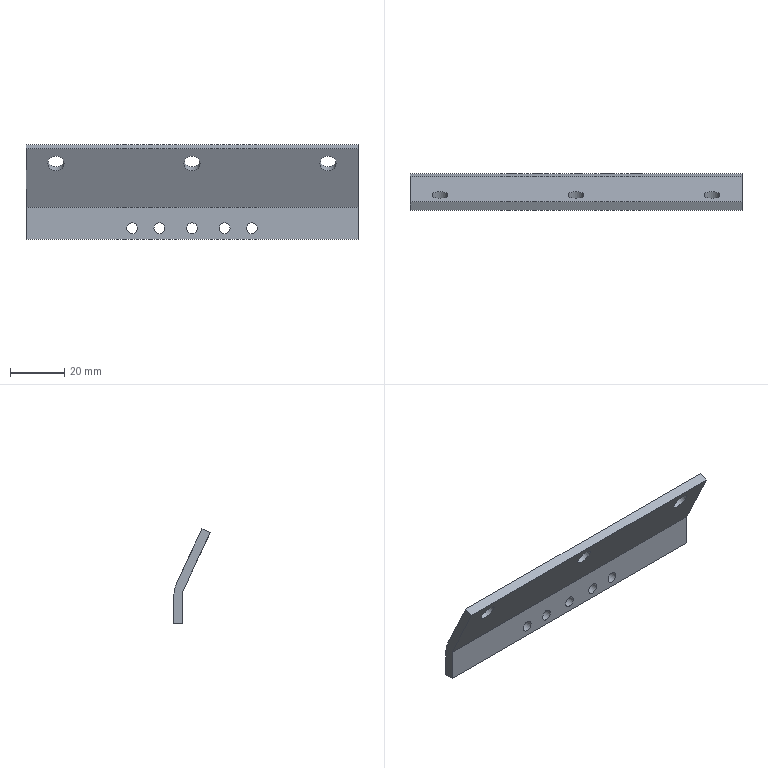Part | STEP file | 1-68.1 | 1 solid | 17 faces | box 122 x 13.367 x 34.723 mm | volume 14145 mm3 | cylinder 9 | plane 8 | commonest cylinder face diameters 4 x5 6 x3 24 x1
STEP:
#1=CARTESIAN_POINT('',(0.,0.,0.));
#2=DIRECTION('',(0.,0.,1.));
#3=DIRECTION('',(1.,0.,0.));
#4=AXIS2_PLACEMENT_3D('',#1,#2,#3);
#5=CARTESIAN_POINT('',(-61.,0.,0.));
#6=VERTEX_POINT('',#5);
#7=CARTESIAN_POINT('',(-61.,3.32,0.));
#8=VERTEX_POINT('',#7);
#9=CARTESIAN_POINT('',(-61.,0.,0.));
#10=DIRECTION('',(0.,1.,0.));
#11=VECTOR('',#10,1.);
#12=LINE('',#9,#11);
#13=CARTESIAN_POINT('',(-61.,7.314,17.361));
#14=DIRECTION('',(1.,0.,0.));
#15=DIRECTION('',(0.,1.,0.));
#16=AXIS2_PLACEMENT_3D('',#13,#14,#15);
#17=PLANE('',#16);
#18=CARTESIAN_POINT('',(-7.314,-17.361));
#19=DIRECTION('',(1.,0.));
#20=VECTOR('',#19,1.);
#21=LINE('',#18,#20);
#22=(GEOMETRIC_REPRESENTATION_CONTEXT(2)PARAMETRIC_REPRESENTATION_CONTEXT()REPRESENTATION_CONTEXT('',''));
#23=DEFINITIONAL_REPRESENTATION('',(#21),#22);
#24=PCURVE('',#17,#23);
#25=CARTESIAN_POINT('',(0.,1.66,0.));
#26=DIRECTION('',(0.,0.,-1.));
#27=DIRECTION('',(0.,1.,0.));
#28=AXIS2_PLACEMENT_3D('',#25,#26,#27);
#29=PLANE('',#28);
#30=CARTESIAN_POINT('',(-1.66,-61.));
#31=DIRECTION('',(1.,0.));
#32=VECTOR('',#31,1.);
#33=LINE('',#30,#32);
#34=(GEOMETRIC_REPRESENTATION_CONTEXT(2)PARAMETRIC_REPRESENTATION_CONTEXT()REPRESENTATION_CONTEXT('',''));
#35=DEFINITIONAL_REPRESENTATION('',(#33),#34);
#36=PCURVE('',#29,#35);
#37=SURFACE_CURVE('',#12,(#24,#36),.PCURVE_S1.);
#38=EDGE_CURVE('',#6,#8,#37,.T.);
#39=ORIENTED_EDGE('',*,*,#38,.T.);
#40=CARTESIAN_POINT('',(-61.,3.32,9.849));
#41=VERTEX_POINT('',#40);
#42=CARTESIAN_POINT('',(-61.,3.32,0.));
#43=DIRECTION('',(0.,0.,1.));
#44=VECTOR('',#43,1.);
#45=LINE('',#42,#44);
#46=CARTESIAN_POINT('',(-3.994,-17.361));
#47=DIRECTION('',(0.,1.));
#48=VECTOR('',#47,1.);
#49=LINE('',#46,#48);
#50=(GEOMETRIC_REPRESENTATION_CONTEXT(2)PARAMETRIC_REPRESENTATION_CONTEXT()REPRESENTATION_CONTEXT('',''));
#51=DEFINITIONAL_REPRESENTATION('',(#49),#50);
#52=PCURVE('',#17,#51);
#53=CARTESIAN_POINT('',(0.,3.32,4.925));
#54=DIRECTION('',(0.,1.,0.));
#55=DIRECTION('',(0.,0.,1.));
#56=AXIS2_PLACEMENT_3D('',#53,#54,#55);
#57=PLANE('',#56);
#58=CARTESIAN_POINT('',(-4.925,-61.));
#59=DIRECTION('',(1.,0.));
#60=VECTOR('',#59,1.);
#61=LINE('',#58,#60);
#62=(GEOMETRIC_REPRESENTATION_CONTEXT(2)PARAMETRIC_REPRESENTATION_CONTEXT()REPRESENTATION_CONTEXT('',''));
#63=DEFINITIONAL_REPRESENTATION('',(#61),#62);
#64=PCURVE('',#57,#63);
#65=SURFACE_CURVE('',#45,(#52,#64),.PCURVE_S1.);
#66=EDGE_CURVE('',#8,#41,#65,.T.);
#67=ORIENTED_EDGE('',*,*,#66,.T.);
#68=CARTESIAN_POINT('',(-61.,2.196,14.921));
#69=VERTEX_POINT('',#68);
#70=CARTESIAN_POINT('',(-61.,-8.68,9.849));
#71=DIRECTION('',(1.,0.,0.));
#72=DIRECTION('',(0.,1.,0.));
#73=AXIS2_PLACEMENT_3D('',#70,#71,#72);
#74=CIRCLE('',#73,12.);
#75=CARTESIAN_POINT('',(-15.994,-7.512));
#76=DIRECTION('',(1.,0.));
#77=AXIS2_PLACEMENT_2D('',#75,#76);
#78=CIRCLE('',#77,12.);
#79=(GEOMETRIC_REPRESENTATION_CONTEXT(2)PARAMETRIC_REPRESENTATION_CONTEXT()REPRESENTATION_CONTEXT('',''));
#80=DEFINITIONAL_REPRESENTATION('',(#78),#79);
#81=PCURVE('',#17,#80);
#82=CARTESIAN_POINT('',(-61.,-8.68,9.849));
#83=DIRECTION('',(1.,0.,0.));
#84=DIRECTION('',(0.,1.,0.));
#85=AXIS2_PLACEMENT_3D('',#82,#83,#84);
#86=CYLINDRICAL_SURFACE('',#85,12.);
#87=CARTESIAN_POINT('',(0.,0.));
#88=DIRECTION('',(1.,0.));
#89=VECTOR('',#88,1.);
#90=LINE('',#87,#89);
#91=(GEOMETRIC_REPRESENTATION_CONTEXT(2)PARAMETRIC_REPRESENTATION_CONTEXT()REPRESENTATION_CONTEXT('',''));
#92=DEFINITIONAL_REPRESENTATION('',(#90),#91);
#93=PCURVE('',#86,#92);
#94=SURFACE_CURVE('',#74,(#81,#93),.PCURVE_S1.);
#95=EDGE_CURVE('',#41,#69,#94,.T.);
#96=ORIENTED_EDGE('',*,*,#95,.T.);
#97=CARTESIAN_POINT('',(-61.,-7.038,34.723));
#98=VERTEX_POINT('',#97);
#99=CARTESIAN_POINT('',(-61.,2.196,14.921));
#100=DIRECTION('',(0.,-0.4226,0.9063));
#101=VECTOR('',#100,1.);
#102=LINE('',#99,#101);
#103=CARTESIAN_POINT('',(-5.118,-2.441));
#104=DIRECTION('',(-0.4226,0.9063));
#105=VECTOR('',#104,1.);
#106=LINE('',#103,#105);
#107=(GEOMETRIC_REPRESENTATION_CONTEXT(2)PARAMETRIC_REPRESENTATION_CONTEXT()REPRESENTATION_CONTEXT('',''));
#108=DEFINITIONAL_REPRESENTATION('',(#106),#107);
#109=PCURVE('',#17,#108);
#110=CARTESIAN_POINT('',(0.,-2.421,24.822));
#111=DIRECTION('',(0.,0.9063,0.4226));
#112=DIRECTION('',(0.,-0.4226,0.9063));
#113=AXIS2_PLACEMENT_3D('',#110,#111,#112);
#114=PLANE('',#113);
#115=CARTESIAN_POINT('',(-10.925,-61.));
#116=DIRECTION('',(1.,0.));
#117=VECTOR('',#116,1.);
#118=LINE('',#115,#117);
#119=(GEOMETRIC_REPRESENTATION_CONTEXT(2)PARAMETRIC_REPRESENTATION_CONTEXT()REPRESENTATION_CONTEXT('',''));
#120=DEFINITIONAL_REPRESENTATION('',(#118),#119);
#121=PCURVE('',#114,#120);
#122=SURFACE_CURVE('',#102,(#109,#121),.PCURVE_S1.);
#123=EDGE_CURVE('',#69,#98,#122,.T.);
#124=ORIENTED_EDGE('',*,*,#123,.T.);
#125=CARTESIAN_POINT('',(-61.,-10.047,33.32));
#126=VERTEX_POINT('',#125);
#127=CARTESIAN_POINT('',(-61.,-7.038,34.723));
#128=DIRECTION('',(0.,-0.9063,-0.4226));
#129=VECTOR('',#128,1.);
#130=LINE('',#127,#129);
#131=CARTESIAN_POINT('',(-14.352,17.361));
#132=DIRECTION('',(-0.9063,-0.4226));
#133=VECTOR('',#132,1.);
#134=LINE('',#131,#133);
#135=(GEOMETRIC_REPRESENTATION_CONTEXT(2)PARAMETRIC_REPRESENTATION_CONTEXT()REPRESENTATION_CONTEXT('',''));
#136=DEFINITIONAL_REPRESENTATION('',(#134),#135);
#137=PCURVE('',#17,#136);
#138=CARTESIAN_POINT('',(0.,-8.543,34.021));
#139=DIRECTION('',(0.,-0.4226,0.9063));
#140=DIRECTION('',(0.,-0.9063,-0.4226));
#141=AXIS2_PLACEMENT_3D('',#138,#139,#140);
#142=PLANE('',#141);
#143=CARTESIAN_POINT('',(-1.66,-61.));
#144=DIRECTION('',(1.,0.));
#145=VECTOR('',#144,1.);
#146=LINE('',#143,#145);
#147=(GEOMETRIC_REPRESENTATION_CONTEXT(2)PARAMETRIC_REPRESENTATION_CONTEXT()REPRESENTATION_CONTEXT('',''));
#148=DEFINITIONAL_REPRESENTATION('',(#146),#147);
#149=PCURVE('',#142,#148);
#150=SURFACE_CURVE('',#130,(#137,#149),.PCURVE_S1.);
#151=EDGE_CURVE('',#98,#126,#150,.T.);
#152=ORIENTED_EDGE('',*,*,#151,.T.);
#153=CARTESIAN_POINT('',(-61.,0.,11.774));
#154=VERTEX_POINT('',#153);
#155=CARTESIAN_POINT('',(-61.,-10.047,33.32));
#156=DIRECTION('',(0.,0.4226,-0.9063));
#157=VECTOR('',#156,1.);
#158=LINE('',#155,#157);
#159=CARTESIAN_POINT('',(-17.361,15.958));
#160=DIRECTION('',(0.4226,-0.9063));
#161=VECTOR('',#160,1.);
#162=LINE('',#159,#161);
#163=(GEOMETRIC_REPRESENTATION_CONTEXT(2)PARAMETRIC_REPRESENTATION_CONTEXT()REPRESENTATION_CONTEXT('',''));
#164=DEFINITIONAL_REPRESENTATION('',(#162),#163);
#165=PCURVE('',#17,#164);
#166=CARTESIAN_POINT('',(0.,-5.024,22.547));
#167=DIRECTION('',(0.,-0.9063,-0.4226));
#168=DIRECTION('',(0.,0.4226,-0.9063));
#169=AXIS2_PLACEMENT_3D('',#166,#167,#168);
#170=PLANE('',#169);
#171=CARTESIAN_POINT('',(-11.887,-61.));
#172=DIRECTION('',(1.,0.));
#173=VECTOR('',#172,1.);
#174=LINE('',#171,#173);
#175=(GEOMETRIC_REPRESENTATION_CONTEXT(2)PARAMETRIC_REPRESENTATION_CONTEXT()REPRESENTATION_CONTEXT('',''));
#176=DEFINITIONAL_REPRESENTATION('',(#174),#175);
#177=PCURVE('',#170,#176);
#178=SURFACE_CURVE('',#158,(#165,#177),.PCURVE_S1.);
#179=EDGE_CURVE('',#126,#154,#178,.T.);
#180=ORIENTED_EDGE('',*,*,#179,.T.);
#181=CARTESIAN_POINT('',(-61.,0.,11.774));
#182=DIRECTION('',(0.,0.,-1.));
#183=VECTOR('',#182,1.);
#184=LINE('',#181,#183);
#185=CARTESIAN_POINT('',(-7.314,-5.588));
#186=DIRECTION('',(0.,-1.));
#187=VECTOR('',#186,1.);
#188=LINE('',#185,#187);
#189=(GEOMETRIC_REPRESENTATION_CONTEXT(2)PARAMETRIC_REPRESENTATION_CONTEXT()REPRESENTATION_CONTEXT('',''));
#190=DEFINITIONAL_REPRESENTATION('',(#188),#189);
#191=PCURVE('',#17,#190);
#192=CARTESIAN_POINT('',(0.,0.,5.887));
#193=DIRECTION('',(0.,-1.,0.));
#194=DIRECTION('',(0.,0.,-1.));
#195=AXIS2_PLACEMENT_3D('',#192,#193,#194);
#196=PLANE('',#195);
#197=CARTESIAN_POINT('',(-5.887,-61.));
#198=DIRECTION('',(1.,0.));
#199=VECTOR('',#198,1.);
#200=LINE('',#197,#199);
#201=(GEOMETRIC_REPRESENTATION_CONTEXT(2)PARAMETRIC_REPRESENTATION_CONTEXT()REPRESENTATION_CONTEXT('',''));
#202=DEFINITIONAL_REPRESENTATION('',(#200),#201);
#203=PCURVE('',#196,#202);
#204=SURFACE_CURVE('',#184,(#191,#203),.PCURVE_S1.);
#205=EDGE_CURVE('',#154,#6,#204,.T.);
#206=ORIENTED_EDGE('',*,*,#205,.T.);
#207=EDGE_LOOP('',(#39,#67,#96,#124,#152,#180,#206));
#208=FACE_BOUND('',#207,.F.);
#209=ADVANCED_FACE('',(#208),#17,.F.);
#210=CARTESIAN_POINT('',(61.,0.,0.));
#211=VERTEX_POINT('',#210);
#212=CARTESIAN_POINT('',(61.,3.32,0.));
#213=VERTEX_POINT('',#212);
#214=CARTESIAN_POINT('',(61.,0.,0.));
#215=DIRECTION('',(0.,1.,0.));
#216=VECTOR('',#215,1.);
#217=LINE('',#214,#216);
#218=CARTESIAN_POINT('',(61.,7.314,17.361));
#219=DIRECTION('',(1.,0.,0.));
#220=DIRECTION('',(0.,1.,0.));
#221=AXIS2_PLACEMENT_3D('',#218,#219,#220);
#222=PLANE('',#221);
#223=CARTESIAN_POINT('',(-7.314,-17.361));
#224=DIRECTION('',(1.,0.));
#225=VECTOR('',#224,1.);
#226=LINE('',#223,#225);
#227=(GEOMETRIC_REPRESENTATION_CONTEXT(2)PARAMETRIC_REPRESENTATION_CONTEXT()REPRESENTATION_CONTEXT('',''));
#228=DEFINITIONAL_REPRESENTATION('',(#226),#227);
#229=PCURVE('',#222,#228);
#230=CARTESIAN_POINT('',(-1.66,61.));
#231=DIRECTION('',(1.,0.));
#232=VECTOR('',#231,1.);
#233=LINE('',#230,#232);
#234=(GEOMETRIC_REPRESENTATION_CONTEXT(2)PARAMETRIC_REPRESENTATION_CONTEXT()REPRESENTATION_CONTEXT('',''));
#235=DEFINITIONAL_REPRESENTATION('',(#233),#234);
#236=PCURVE('',#29,#235);
#237=SURFACE_CURVE('',#217,(#229,#236),.PCURVE_S1.);
#238=EDGE_CURVE('',#211,#213,#237,.T.);
#239=ORIENTED_EDGE('',*,*,#238,.T.);
#240=CARTESIAN_POINT('',(61.,3.32,9.849));
#241=VERTEX_POINT('',#240);
#242=CARTESIAN_POINT('',(61.,3.32,0.));
#243=DIRECTION('',(0.,0.,1.));
#244=VECTOR('',#243,1.);
#245=LINE('',#242,#244);
#246=CARTESIAN_POINT('',(-3.994,-17.361));
#247=DIRECTION('',(0.,1.));
#248=VECTOR('',#247,1.);
#249=LINE('',#246,#248);
#250=(GEOMETRIC_REPRESENTATION_CONTEXT(2)PARAMETRIC_REPRESENTATION_CONTEXT()REPRESENTATION_CONTEXT('',''));
#251=DEFINITIONAL_REPRESENTATION('',(#249),#250);
#252=PCURVE('',#222,#251);
#253=CARTESIAN_POINT('',(-4.925,61.));
#254=DIRECTION('',(1.,0.));
#255=VECTOR('',#254,1.);
#256=LINE('',#253,#255);
#257=(GEOMETRIC_REPRESENTATION_CONTEXT(2)PARAMETRIC_REPRESENTATION_CONTEXT()REPRESENTATION_CONTEXT('',''));
#258=DEFINITIONAL_REPRESENTATION('',(#256),#257);
#259=PCURVE('',#57,#258);
#260=SURFACE_CURVE('',#245,(#252,#259),.PCURVE_S1.);
#261=EDGE_CURVE('',#213,#241,#260,.T.);
#262=ORIENTED_EDGE('',*,*,#261,.T.);
#263=CARTESIAN_POINT('',(61.,2.196,14.921));
#264=VERTEX_POINT('',#263);
#265=CARTESIAN_POINT('',(61.,-8.68,9.849));
#266=DIRECTION('',(1.,0.,0.));
#267=DIRECTION('',(0.,1.,0.));
#268=AXIS2_PLACEMENT_3D('',#265,#266,#267);
#269=CIRCLE('',#268,12.);
#270=CARTESIAN_POINT('',(-15.994,-7.512));
#271=DIRECTION('',(1.,0.));
#272=AXIS2_PLACEMENT_2D('',#270,#271);
#273=CIRCLE('',#272,12.);
#274=(GEOMETRIC_REPRESENTATION_CONTEXT(2)PARAMETRIC_REPRESENTATION_CONTEXT()REPRESENTATION_CONTEXT('',''));
#275=DEFINITIONAL_REPRESENTATION('',(#273),#274);
#276=PCURVE('',#222,#275);
#277=CARTESIAN_POINT('',(0.,122.));
#278=DIRECTION('',(1.,0.));
#279=VECTOR('',#278,1.);
#280=LINE('',#277,#279);
#281=(GEOMETRIC_REPRESENTATION_CONTEXT(2)PARAMETRIC_REPRESENTATION_CONTEXT()REPRESENTATION_CONTEXT('',''));
#282=DEFINITIONAL_REPRESENTATION('',(#280),#281);
#283=PCURVE('',#86,#282);
#284=SURFACE_CURVE('',#269,(#276,#283),.PCURVE_S1.);
#285=EDGE_CURVE('',#241,#264,#284,.T.);
#286=ORIENTED_EDGE('',*,*,#285,.T.);
#287=CARTESIAN_POINT('',(61.,-7.038,34.723));
#288=VERTEX_POINT('',#287);
#289=CARTESIAN_POINT('',(61.,2.196,14.921));
#290=DIRECTION('',(0.,-0.4226,0.9063));
#291=VECTOR('',#290,1.);
#292=LINE('',#289,#291);
#293=CARTESIAN_POINT('',(-5.118,-2.441));
#294=DIRECTION('',(-0.4226,0.9063));
#295=VECTOR('',#294,1.);
#296=LINE('',#293,#295);
#297=(GEOMETRIC_REPRESENTATION_CONTEXT(2)PARAMETRIC_REPRESENTATION_CONTEXT()REPRESENTATION_CONTEXT('',''));
#298=DEFINITIONAL_REPRESENTATION('',(#296),#297);
#299=PCURVE('',#222,#298);
#300=CARTESIAN_POINT('',(-10.925,61.));
#301=DIRECTION('',(1.,0.));
#302=VECTOR('',#301,1.);
#303=LINE('',#300,#302);
#304=(GEOMETRIC_REPRESENTATION_CONTEXT(2)PARAMETRIC_REPRESENTATION_CONTEXT()REPRESENTATION_CONTEXT('',''));
#305=DEFINITIONAL_REPRESENTATION('',(#303),#304);
#306=PCURVE('',#114,#305);
#307=SURFACE_CURVE('',#292,(#299,#306),.PCURVE_S1.);
#308=EDGE_CURVE('',#264,#288,#307,.T.);
#309=ORIENTED_EDGE('',*,*,#308,.T.);
#310=CARTESIAN_POINT('',(61.,-10.047,33.32));
#311=VERTEX_POINT('',#310);
#312=CARTESIAN_POINT('',(61.,-7.038,34.723));
#313=DIRECTION('',(0.,-0.9063,-0.4226));
#314=VECTOR('',#313,1.);
#315=LINE('',#312,#314);
#316=CARTESIAN_POINT('',(-14.352,17.361));
#317=DIRECTION('',(-0.9063,-0.4226));
#318=VECTOR('',#317,1.);
#319=LINE('',#316,#318);
#320=(GEOMETRIC_REPRESENTATION_CONTEXT(2)PARAMETRIC_REPRESENTATION_CONTEXT()REPRESENTATION_CONTEXT('',''));
#321=DEFINITIONAL_REPRESENTATION('',(#319),#320);
#322=PCURVE('',#222,#321);
#323=CARTESIAN_POINT('',(-1.66,61.));
#324=DIRECTION('',(1.,0.));
#325=VECTOR('',#324,1.);
#326=LINE('',#323,#325);
#327=(GEOMETRIC_REPRESENTATION_CONTEXT(2)PARAMETRIC_REPRESENTATION_CONTEXT()REPRESENTATION_CONTEXT('',''));
#328=DEFINITIONAL_REPRESENTATION('',(#326),#327);
#329=PCURVE('',#142,#328);
#330=SURFACE_CURVE('',#315,(#322,#329),.PCURVE_S1.);
#331=EDGE_CURVE('',#288,#311,#330,.T.);
#332=ORIENTED_EDGE('',*,*,#331,.T.);
#333=CARTESIAN_POINT('',(61.,0.,11.774));
#334=VERTEX_POINT('',#333);
#335=CARTESIAN_POINT('',(61.,-10.047,33.32));
#336=DIRECTION('',(0.,0.4226,-0.9063));
#337=VECTOR('',#336,1.);
#338=LINE('',#335,#337);
#339=CARTESIAN_POINT('',(-17.361,15.958));
#340=DIRECTION('',(0.4226,-0.9063));
#341=VECTOR('',#340,1.);
#342=LINE('',#339,#341);
#343=(GEOMETRIC_REPRESENTATION_CONTEXT(2)PARAMETRIC_REPRESENTATION_CONTEXT()REPRESENTATION_CONTEXT('',''));
#344=DEFINITIONAL_REPRESENTATION('',(#342),#343);
#345=PCURVE('',#222,#344);
#346=CARTESIAN_POINT('',(-11.887,61.));
#347=DIRECTION('',(1.,0.));
#348=VECTOR('',#347,1.);
#349=LINE('',#346,#348);
#350=(GEOMETRIC_REPRESENTATION_CONTEXT(2)PARAMETRIC_REPRESENTATION_CONTEXT()REPRESENTATION_CONTEXT('',''));
#351=DEFINITIONAL_REPRESENTATION('',(#349),#350);
#352=PCURVE('',#170,#351);
#353=SURFACE_CURVE('',#338,(#345,#352),.PCURVE_S1.);
#354=EDGE_CURVE('',#311,#334,#353,.T.);
#355=ORIENTED_EDGE('',*,*,#354,.T.);
#356=CARTESIAN_POINT('',(61.,0.,11.774));
#357=DIRECTION('',(0.,0.,-1.));
#358=VECTOR('',#357,1.);
#359=LINE('',#356,#358);
#360=CARTESIAN_POINT('',(-7.314,-5.588));
#361=DIRECTION('',(0.,-1.));
#362=VECTOR('',#361,1.);
#363=LINE('',#360,#362);
#364=(GEOMETRIC_REPRESENTATION_CONTEXT(2)PARAMETRIC_REPRESENTATION_CONTEXT()REPRESENTATION_CONTEXT('',''));
#365=DEFINITIONAL_REPRESENTATION('',(#363),#364);
#366=PCURVE('',#222,#365);
#367=CARTESIAN_POINT('',(-5.887,61.));
#368=DIRECTION('',(1.,0.));
#369=VECTOR('',#368,1.);
#370=LINE('',#367,#369);
#371=(GEOMETRIC_REPRESENTATION_CONTEXT(2)PARAMETRIC_REPRESENTATION_CONTEXT()REPRESENTATION_CONTEXT('',''));
#372=DEFINITIONAL_REPRESENTATION('',(#370),#371);
#373=PCURVE('',#196,#372);
#374=SURFACE_CURVE('',#359,(#366,#373),.PCURVE_S1.);
#375=EDGE_CURVE('',#334,#211,#374,.T.);
#376=ORIENTED_EDGE('',*,*,#375,.T.);
#377=EDGE_LOOP('',(#239,#262,#286,#309,#332,#355,#376));
#378=FACE_BOUND('',#377,.T.);
#379=ADVANCED_FACE('',(#378),#222,.T.);
#380=ORIENTED_EDGE('',*,*,#38,.T.);
#381=CARTESIAN_POINT('',(-61.,3.32,0.));
#382=DIRECTION('',(1.,0.,0.));
#383=VECTOR('',#382,1.);
#384=LINE('',#381,#383);
#385=CARTESIAN_POINT('',(1.66,-61.));
#386=DIRECTION('',(0.,1.));
#387=VECTOR('',#386,1.);
#388=LINE('',#385,#387);
#389=(GEOMETRIC_REPRESENTATION_CONTEXT(2)PARAMETRIC_REPRESENTATION_CONTEXT()REPRESENTATION_CONTEXT('',''));
#390=DEFINITIONAL_REPRESENTATION('',(#388),#389);
#391=PCURVE('',#29,#390);
#392=CARTESIAN_POINT('',(-4.925,-61.));
#393=DIRECTION('',(0.,1.));
#394=VECTOR('',#393,1.);
#395=LINE('',#392,#394);
#396=(GEOMETRIC_REPRESENTATION_CONTEXT(2)PARAMETRIC_REPRESENTATION_CONTEXT()REPRESENTATION_CONTEXT('',''));
#397=DEFINITIONAL_REPRESENTATION('',(#395),#396);
#398=PCURVE('',#57,#397);
#399=SURFACE_CURVE('',#384,(#391,#398),.PCURVE_S1.);
#400=EDGE_CURVE('',#8,#213,#399,.T.);
#401=ORIENTED_EDGE('',*,*,#400,.T.);
#402=ORIENTED_EDGE('',*,*,#238,.F.);
#403=CARTESIAN_POINT('',(-61.,0.,0.));
#404=DIRECTION('',(1.,0.,0.));
#405=VECTOR('',#404,1.);
#406=LINE('',#403,#405);
#407=CARTESIAN_POINT('',(-1.66,-61.));
#408=DIRECTION('',(0.,1.));
#409=VECTOR('',#408,1.);
#410=LINE('',#407,#409);
#411=(GEOMETRIC_REPRESENTATION_CONTEXT(2)PARAMETRIC_REPRESENTATION_CONTEXT()REPRESENTATION_CONTEXT('',''));
#412=DEFINITIONAL_REPRESENTATION('',(#410),#411);
#413=PCURVE('',#29,#412);
#414=CARTESIAN_POINT('',(5.887,-61.));
#415=DIRECTION('',(0.,1.));
#416=VECTOR('',#415,1.);
#417=LINE('',#414,#416);
#418=(GEOMETRIC_REPRESENTATION_CONTEXT(2)PARAMETRIC_REPRESENTATION_CONTEXT()REPRESENTATION_CONTEXT('',''));
#419=DEFINITIONAL_REPRESENTATION('',(#417),#418);
#420=PCURVE('',#196,#419);
#421=SURFACE_CURVE('',#406,(#413,#420),.PCURVE_S1.);
#422=EDGE_CURVE('',#6,#211,#421,.T.);
#423=ORIENTED_EDGE('',*,*,#422,.F.);
#424=EDGE_LOOP('',(#380,#401,#402,#423));
#425=FACE_BOUND('',#424,.T.);
#426=ADVANCED_FACE('',(#425),#29,.T.);
#427=ORIENTED_EDGE('',*,*,#95,.T.);
#428=CARTESIAN_POINT('',(-61.,2.196,14.921));
#429=DIRECTION('',(1.,0.,0.));
#430=VECTOR('',#429,1.);
#431=LINE('',#428,#430);
#432=CARTESIAN_POINT('',(0.4363,0.));
#433=DIRECTION('',(0.,1.));
#434=VECTOR('',#433,1.);
#435=LINE('',#432,#434);
#436=(GEOMETRIC_REPRESENTATION_CONTEXT(2)PARAMETRIC_REPRESENTATION_CONTEXT()REPRESENTATION_CONTEXT('',''));
#437=DEFINITIONAL_REPRESENTATION('',(#435),#436);
#438=PCURVE('',#86,#437);
#439=CARTESIAN_POINT('',(-10.925,-61.));
#440=DIRECTION('',(0.,1.));
#441=VECTOR('',#440,1.);
#442=LINE('',#439,#441);
#443=(GEOMETRIC_REPRESENTATION_CONTEXT(2)PARAMETRIC_REPRESENTATION_CONTEXT()REPRESENTATION_CONTEXT('',''));
#444=DEFINITIONAL_REPRESENTATION('',(#442),#443);
#445=PCURVE('',#114,#444);
#446=SURFACE_CURVE('',#431,(#438,#445),.PCURVE_S1.);
#447=EDGE_CURVE('',#69,#264,#446,.T.);
#448=ORIENTED_EDGE('',*,*,#447,.T.);
#449=ORIENTED_EDGE('',*,*,#285,.F.);
#450=CARTESIAN_POINT('',(-61.,3.32,9.849));
#451=DIRECTION('',(1.,0.,0.));
#452=VECTOR('',#451,1.);
#453=LINE('',#450,#452);
#454=CARTESIAN_POINT('',(0.,0.));
#455=DIRECTION('',(0.,1.));
#456=VECTOR('',#455,1.);
#457=LINE('',#454,#456);
#458=(GEOMETRIC_REPRESENTATION_CONTEXT(2)PARAMETRIC_REPRESENTATION_CONTEXT()REPRESENTATION_CONTEXT('',''));
#459=DEFINITIONAL_REPRESENTATION('',(#457),#458);
#460=PCURVE('',#86,#459);
#461=CARTESIAN_POINT('',(4.925,-61.));
#462=DIRECTION('',(0.,1.));
#463=VECTOR('',#462,1.);
#464=LINE('',#461,#463);
#465=(GEOMETRIC_REPRESENTATION_CONTEXT(2)PARAMETRIC_REPRESENTATION_CONTEXT()REPRESENTATION_CONTEXT('',''));
#466=DEFINITIONAL_REPRESENTATION('',(#464),#465);
#467=PCURVE('',#57,#466);
#468=SURFACE_CURVE('',#453,(#460,#467),.PCURVE_S1.);
#469=EDGE_CURVE('',#41,#241,#468,.T.);
#470=ORIENTED_EDGE('',*,*,#469,.F.);
#471=EDGE_LOOP('',(#427,#448,#449,#470));
#472=FACE_BOUND('',#471,.T.);
#473=ADVANCED_FACE('',(#472),#86,.T.);
#474=ORIENTED_EDGE('',*,*,#151,.T.);
#475=CARTESIAN_POINT('',(-61.,-10.047,33.32));
#476=DIRECTION('',(1.,0.,0.));
#477=VECTOR('',#476,1.);
#478=LINE('',#475,#477);
#479=CARTESIAN_POINT('',(1.66,-61.));
#480=DIRECTION('',(0.,1.));
#481=VECTOR('',#480,1.);
#482=LINE('',#479,#481);
#483=(GEOMETRIC_REPRESENTATION_CONTEXT(2)PARAMETRIC_REPRESENTATION_CONTEXT()REPRESENTATION_CONTEXT('',''));
#484=DEFINITIONAL_REPRESENTATION('',(#482),#483);
#485=PCURVE('',#142,#484);
#486=CARTESIAN_POINT('',(-11.887,-61.));
#487=DIRECTION('',(0.,1.));
#488=VECTOR('',#487,1.);
#489=LINE('',#486,#488);
#490=(GEOMETRIC_REPRESENTATION_CONTEXT(2)PARAMETRIC_REPRESENTATION_CONTEXT()REPRESENTATION_CONTEXT('',''));
#491=DEFINITIONAL_REPRESENTATION('',(#489),#490);
#492=PCURVE('',#170,#491);
#493=SURFACE_CURVE('',#478,(#485,#492),.PCURVE_S1.);
#494=EDGE_CURVE('',#126,#311,#493,.T.);
#495=ORIENTED_EDGE('',*,*,#494,.T.);
#496=ORIENTED_EDGE('',*,*,#331,.F.);
#497=CARTESIAN_POINT('',(-61.,-7.038,34.723));
#498=DIRECTION('',(1.,0.,0.));
#499=VECTOR('',#498,1.);
#500=LINE('',#497,#499);
#501=CARTESIAN_POINT('',(-1.66,-61.));
#502=DIRECTION('',(0.,1.));
#503=VECTOR('',#502,1.);
#504=LINE('',#501,#503);
#505=(GEOMETRIC_REPRESENTATION_CONTEXT(2)PARAMETRIC_REPRESENTATION_CONTEXT()REPRESENTATION_CONTEXT('',''));
#506=DEFINITIONAL_REPRESENTATION('',(#504),#505);
#507=PCURVE('',#142,#506);
#508=CARTESIAN_POINT('',(10.925,-61.));
#509=DIRECTION('',(0.,1.));
#510=VECTOR('',#509,1.);
#511=LINE('',#508,#510);
#512=(GEOMETRIC_REPRESENTATION_CONTEXT(2)PARAMETRIC_REPRESENTATION_CONTEXT()REPRESENTATION_CONTEXT('',''));
#513=DEFINITIONAL_REPRESENTATION('',(#511),#512);
#514=PCURVE('',#114,#513);
#515=SURFACE_CURVE('',#500,(#507,#514),.PCURVE_S1.);
#516=EDGE_CURVE('',#98,#288,#515,.T.);
#517=ORIENTED_EDGE('',*,*,#516,.F.);
#518=EDGE_LOOP('',(#474,#495,#496,#517));
#519=FACE_BOUND('',#518,.T.);
#520=ADVANCED_FACE('',(#519),#142,.T.);
#521=ORIENTED_EDGE('',*,*,#123,.T.);
#522=ORIENTED_EDGE('',*,*,#516,.T.);
#523=ORIENTED_EDGE('',*,*,#308,.F.);
#524=ORIENTED_EDGE('',*,*,#447,.F.);
#525=EDGE_LOOP('',(#521,#522,#523,#524));
#526=FACE_BOUND('',#525,.T.);
#527=CARTESIAN_POINT('',(47.,-4.502,29.285));
#528=VERTEX_POINT('',#527);
#529=CARTESIAN_POINT('',(50.,-4.502,29.285));
#530=DIRECTION('',(0.,0.9063,0.4226));
#531=DIRECTION('',(-1.,0.,0.));
#532=AXIS2_PLACEMENT_3D('',#529,#530,#531);
#533=CIRCLE('',#532,3.);
#534=CARTESIAN_POINT('',(4.925,50.));
#535=DIRECTION('',(0.,-1.));
#536=AXIS2_PLACEMENT_2D('',#534,#535);
#537=CIRCLE('',#536,3.);
#538=(GEOMETRIC_REPRESENTATION_CONTEXT(2)PARAMETRIC_REPRESENTATION_CONTEXT()REPRESENTATION_CONTEXT('',''));
#539=DEFINITIONAL_REPRESENTATION('',(#537),#538);
#540=PCURVE('',#114,#539);
#541=CARTESIAN_POINT('',(50.,-59.787,3.505));
#542=DIRECTION('',(0.,0.9063,0.4226));
#543=DIRECTION('',(-1.,0.,0.));
#544=AXIS2_PLACEMENT_3D('',#541,#542,#543);
#545=CYLINDRICAL_SURFACE('',#544,3.);
#546=CARTESIAN_POINT('',(0.,61.));
#547=DIRECTION('',(1.,0.));
#548=VECTOR('',#547,1.);
#549=LINE('',#546,#548);
#550=(GEOMETRIC_REPRESENTATION_CONTEXT(2)PARAMETRIC_REPRESENTATION_CONTEXT()REPRESENTATION_CONTEXT('',''));
#551=DEFINITIONAL_REPRESENTATION('',(#549),#550);
#552=PCURVE('',#545,#551);
#553=SURFACE_CURVE('',#533,(#540,#552),.PCURVE_S1.);
#554=EDGE_CURVE('',#528,#528,#553,.T.);
#555=ORIENTED_EDGE('',*,*,#554,.F.);
#556=EDGE_LOOP('',(#555));
#557=FACE_BOUND('',#556,.T.);
#558=CARTESIAN_POINT('',(-3.,-4.502,29.285));
#559=VERTEX_POINT('',#558);
#560=CARTESIAN_POINT('',(0.,-4.502,29.285));
#561=DIRECTION('',(0.,0.9063,0.4226));
#562=DIRECTION('',(-1.,0.,0.));
#563=AXIS2_PLACEMENT_3D('',#560,#561,#562);
#564=CIRCLE('',#563,3.);
#565=CARTESIAN_POINT('',(4.925,0.));
#566=DIRECTION('',(0.,-1.));
#567=AXIS2_PLACEMENT_2D('',#565,#566);
#568=CIRCLE('',#567,3.);
#569=(GEOMETRIC_REPRESENTATION_CONTEXT(2)PARAMETRIC_REPRESENTATION_CONTEXT()REPRESENTATION_CONTEXT('',''));
#570=DEFINITIONAL_REPRESENTATION('',(#568),#569);
#571=PCURVE('',#114,#570);
#572=CARTESIAN_POINT('',(0.,-59.787,3.505));
#573=DIRECTION('',(0.,0.9063,0.4226));
#574=DIRECTION('',(-1.,0.,0.));
#575=AXIS2_PLACEMENT_3D('',#572,#573,#574);
#576=CYLINDRICAL_SURFACE('',#575,3.);
#577=CARTESIAN_POINT('',(0.,61.));
#578=DIRECTION('',(1.,0.));
#579=VECTOR('',#578,1.);
#580=LINE('',#577,#579);
#581=(GEOMETRIC_REPRESENTATION_CONTEXT(2)PARAMETRIC_REPRESENTATION_CONTEXT()REPRESENTATION_CONTEXT('',''));
#582=DEFINITIONAL_REPRESENTATION('',(#580),#581);
#583=PCURVE('',#576,#582);
#584=SURFACE_CURVE('',#564,(#571,#583),.PCURVE_S1.);
#585=EDGE_CURVE('',#559,#559,#584,.T.);
#586=ORIENTED_EDGE('',*,*,#585,.F.);
#587=EDGE_LOOP('',(#586));
#588=FACE_BOUND('',#587,.T.);
#589=CARTESIAN_POINT('',(-53.,-4.502,29.285));
#590=VERTEX_POINT('',#589);
#591=CARTESIAN_POINT('',(-50.,-4.502,29.285));
#592=DIRECTION('',(0.,0.9063,0.4226));
#593=DIRECTION('',(-1.,0.,0.));
#594=AXIS2_PLACEMENT_3D('',#591,#592,#593);
#595=CIRCLE('',#594,3.);
#596=CARTESIAN_POINT('',(4.925,-50.));
#597=DIRECTION('',(0.,-1.));
#598=AXIS2_PLACEMENT_2D('',#596,#597);
#599=CIRCLE('',#598,3.);
#600=(GEOMETRIC_REPRESENTATION_CONTEXT(2)PARAMETRIC_REPRESENTATION_CONTEXT()REPRESENTATION_CONTEXT('',''));
#601=DEFINITIONAL_REPRESENTATION('',(#599),#600);
#602=PCURVE('',#114,#601);
#603=CARTESIAN_POINT('',(-50.,-59.787,3.505));
#604=DIRECTION('',(0.,0.9063,0.4226));
#605=DIRECTION('',(-1.,0.,0.));
#606=AXIS2_PLACEMENT_3D('',#603,#604,#605);
#607=CYLINDRICAL_SURFACE('',#606,3.);
#608=CARTESIAN_POINT('',(0.,61.));
#609=DIRECTION('',(1.,0.));
#610=VECTOR('',#609,1.);
#611=LINE('',#608,#610);
#612=(GEOMETRIC_REPRESENTATION_CONTEXT(2)PARAMETRIC_REPRESENTATION_CONTEXT()REPRESENTATION_CONTEXT('',''));
#613=DEFINITIONAL_REPRESENTATION('',(#611),#612);
#614=PCURVE('',#607,#613);
#615=SURFACE_CURVE('',#595,(#602,#614),.PCURVE_S1.);
#616=EDGE_CURVE('',#590,#590,#615,.T.);
#617=ORIENTED_EDGE('',*,*,#616,.F.);
#618=EDGE_LOOP('',(#617));
#619=FACE_BOUND('',#618,.T.);
#620=ADVANCED_FACE('',(#526,#557,#588,#619),#114,.T.);
#621=ORIENTED_EDGE('',*,*,#179,.T.);
#622=CARTESIAN_POINT('',(-61.,0.,11.774));
#623=DIRECTION('',(1.,0.,0.));
#624=VECTOR('',#623,1.);
#625=LINE('',#622,#624);
#626=CARTESIAN_POINT('',(11.887,-61.));
#627=DIRECTION('',(0.,1.));
#628=VECTOR('',#627,1.);
#629=LINE('',#626,#628);
#630=(GEOMETRIC_REPRESENTATION_CONTEXT(2)PARAMETRIC_REPRESENTATION_CONTEXT()REPRESENTATION_CONTEXT('',''));
#631=DEFINITIONAL_REPRESENTATION('',(#629),#630);
#632=PCURVE('',#170,#631);
#633=CARTESIAN_POINT('',(-5.887,-61.));
#634=DIRECTION('',(0.,1.));
#635=VECTOR('',#634,1.);
#636=LINE('',#633,#635);
#637=(GEOMETRIC_REPRESENTATION_CONTEXT(2)PARAMETRIC_REPRESENTATION_CONTEXT()REPRESENTATION_CONTEXT('',''));
#638=DEFINITIONAL_REPRESENTATION('',(#636),#637);
#639=PCURVE('',#196,#638);
#640=SURFACE_CURVE('',#625,(#632,#639),.PCURVE_S1.);
#641=EDGE_CURVE('',#154,#334,#640,.T.);
#642=ORIENTED_EDGE('',*,*,#641,.T.);
#643=ORIENTED_EDGE('',*,*,#354,.F.);
#644=ORIENTED_EDGE('',*,*,#494,.F.);
#645=EDGE_LOOP('',(#621,#642,#643,#644));
#646=FACE_BOUND('',#645,.T.);
#647=CARTESIAN_POINT('',(47.,-7.511,27.882));
#648=VERTEX_POINT('',#647);
#649=CARTESIAN_POINT('',(50.,-7.511,27.882));
#650=DIRECTION('',(0.,-0.9063,-0.4226));
#651=DIRECTION('',(-1.,0.,0.));
#652=AXIS2_PLACEMENT_3D('',#649,#650,#651);
#653=CIRCLE('',#652,3.);
#654=CARTESIAN_POINT('',(-5.887,50.));
#655=DIRECTION('',(0.,-1.));
#656=AXIS2_PLACEMENT_2D('',#654,#655);
#657=CIRCLE('',#656,3.);
#658=(GEOMETRIC_REPRESENTATION_CONTEXT(2)PARAMETRIC_REPRESENTATION_CONTEXT()REPRESENTATION_CONTEXT('',''));
#659=DEFINITIONAL_REPRESENTATION('',(#657),#658);
#660=PCURVE('',#170,#659);
#661=CARTESIAN_POINT('',(6.283,57.68));
#662=DIRECTION('',(-1.,0.));
#663=VECTOR('',#662,1.);
#664=LINE('',#661,#663);
#665=(GEOMETRIC_REPRESENTATION_CONTEXT(2)PARAMETRIC_REPRESENTATION_CONTEXT()REPRESENTATION_CONTEXT('',''));
#666=DEFINITIONAL_REPRESENTATION('',(#664),#665);
#667=PCURVE('',#545,#666);
#668=SURFACE_CURVE('',#653,(#660,#667),.PCURVE_S1.);
#669=EDGE_CURVE('',#648,#648,#668,.T.);
#670=ORIENTED_EDGE('',*,*,#669,.F.);
#671=EDGE_LOOP('',(#670));
#672=FACE_BOUND('',#671,.T.);
#673=CARTESIAN_POINT('',(-3.,-7.511,27.882));
#674=VERTEX_POINT('',#673);
#675=CARTESIAN_POINT('',(0.,-7.511,27.882));
#676=DIRECTION('',(0.,-0.9063,-0.4226));
#677=DIRECTION('',(-1.,0.,0.));
#678=AXIS2_PLACEMENT_3D('',#675,#676,#677);
#679=CIRCLE('',#678,3.);
#680=CARTESIAN_POINT('',(-5.887,0.));
#681=DIRECTION('',(0.,-1.));
#682=AXIS2_PLACEMENT_2D('',#680,#681);
#683=CIRCLE('',#682,3.);
#684=(GEOMETRIC_REPRESENTATION_CONTEXT(2)PARAMETRIC_REPRESENTATION_CONTEXT()REPRESENTATION_CONTEXT('',''));
#685=DEFINITIONAL_REPRESENTATION('',(#683),#684);
#686=PCURVE('',#170,#685);
#687=CARTESIAN_POINT('',(6.283,57.68));
#688=DIRECTION('',(-1.,0.));
#689=VECTOR('',#688,1.);
#690=LINE('',#687,#689);
#691=(GEOMETRIC_REPRESENTATION_CONTEXT(2)PARAMETRIC_REPRESENTATION_CONTEXT()REPRESENTATION_CONTEXT('',''));
#692=DEFINITIONAL_REPRESENTATION('',(#690),#691);
#693=PCURVE('',#576,#692);
#694=SURFACE_CURVE('',#679,(#686,#693),.PCURVE_S1.);
#695=EDGE_CURVE('',#674,#674,#694,.T.);
#696=ORIENTED_EDGE('',*,*,#695,.F.);
#697=EDGE_LOOP('',(#696));
#698=FACE_BOUND('',#697,.T.);
#699=CARTESIAN_POINT('',(-53.,-7.511,27.882));
#700=VERTEX_POINT('',#699);
#701=CARTESIAN_POINT('',(-50.,-7.511,27.882));
#702=DIRECTION('',(0.,-0.9063,-0.4226));
#703=DIRECTION('',(-1.,0.,0.));
#704=AXIS2_PLACEMENT_3D('',#701,#702,#703);
#705=CIRCLE('',#704,3.);
#706=CARTESIAN_POINT('',(-5.887,-50.));
#707=DIRECTION('',(0.,-1.));
#708=AXIS2_PLACEMENT_2D('',#706,#707);
#709=CIRCLE('',#708,3.);
#710=(GEOMETRIC_REPRESENTATION_CONTEXT(2)PARAMETRIC_REPRESENTATION_CONTEXT()REPRESENTATION_CONTEXT('',''));
#711=DEFINITIONAL_REPRESENTATION('',(#709),#710);
#712=PCURVE('',#170,#711);
#713=CARTESIAN_POINT('',(6.283,57.68));
#714=DIRECTION('',(-1.,0.));
#715=VECTOR('',#714,1.);
#716=LINE('',#713,#715);
#717=(GEOMETRIC_REPRESENTATION_CONTEXT(2)PARAMETRIC_REPRESENTATION_CONTEXT()REPRESENTATION_CONTEXT('',''));
#718=DEFINITIONAL_REPRESENTATION('',(#716),#717);
#719=PCURVE('',#607,#718);
#720=SURFACE_CURVE('',#705,(#712,#719),.PCURVE_S1.);
#721=EDGE_CURVE('',#700,#700,#720,.T.);
#722=ORIENTED_EDGE('',*,*,#721,.F.);
#723=EDGE_LOOP('',(#722));
#724=FACE_BOUND('',#723,.T.);
#725=ADVANCED_FACE('',(#646,#672,#698,#724),#170,.T.);
#726=CARTESIAN_POINT('',(47.,-7.511,27.882));
#727=DIRECTION('',(0.,0.9063,0.4226));
#728=VECTOR('',#727,1.);
#729=LINE('',#726,#728);
#730=CARTESIAN_POINT('',(0.,57.68));
#731=DIRECTION('',(0.,1.));
#732=VECTOR('',#731,1.);
#733=LINE('',#730,#732);
#734=(GEOMETRIC_REPRESENTATION_CONTEXT(2)PARAMETRIC_REPRESENTATION_CONTEXT()REPRESENTATION_CONTEXT('',''));
#735=DEFINITIONAL_REPRESENTATION('',(#733),#734);
#736=PCURVE('',#545,#735);
#737=CARTESIAN_POINT('',(6.283,57.68));
#738=DIRECTION('',(0.,1.));
#739=VECTOR('',#738,1.);
#740=LINE('',#737,#739);
#741=(GEOMETRIC_REPRESENTATION_CONTEXT(2)PARAMETRIC_REPRESENTATION_CONTEXT()REPRESENTATION_CONTEXT('',''));
#742=DEFINITIONAL_REPRESENTATION('',(#740),#741);
#743=PCURVE('',#545,#742);
#744=SEAM_CURVE('',#729,(#736,#743),.PCURVE_S1.);
#745=EDGE_CURVE('',#648,#528,#744,.T.);
#746=ORIENTED_EDGE('',*,*,#745,.F.);
#747=ORIENTED_EDGE('',*,*,#669,.F.);
#748=ORIENTED_EDGE('',*,*,#745,.T.);
#749=ORIENTED_EDGE('',*,*,#554,.F.);
#750=EDGE_LOOP('',(#746,#747,#748,#749));
#751=FACE_BOUND('',#750,.F.);
#752=ADVANCED_FACE('',(#751),#545,.F.);
#753=CARTESIAN_POINT('',(-3.,-7.511,27.882));
#754=DIRECTION('',(0.,0.9063,0.4226));
#755=VECTOR('',#754,1.);
#756=LINE('',#753,#755);
#757=CARTESIAN_POINT('',(0.,57.68));
#758=DIRECTION('',(0.,1.));
#759=VECTOR('',#758,1.);
#760=LINE('',#757,#759);
#761=(GEOMETRIC_REPRESENTATION_CONTEXT(2)PARAMETRIC_REPRESENTATION_CONTEXT()REPRESENTATION_CONTEXT('',''));
#762=DEFINITIONAL_REPRESENTATION('',(#760),#761);
#763=PCURVE('',#576,#762);
#764=CARTESIAN_POINT('',(6.283,57.68));
#765=DIRECTION('',(0.,1.));
#766=VECTOR('',#765,1.);
#767=LINE('',#764,#766);
#768=(GEOMETRIC_REPRESENTATION_CONTEXT(2)PARAMETRIC_REPRESENTATION_CONTEXT()REPRESENTATION_CONTEXT('',''));
#769=DEFINITIONAL_REPRESENTATION('',(#767),#768);
#770=PCURVE('',#576,#769);
#771=SEAM_CURVE('',#756,(#763,#770),.PCURVE_S1.);
#772=EDGE_CURVE('',#674,#559,#771,.T.);
#773=ORIENTED_EDGE('',*,*,#772,.F.);
#774=ORIENTED_EDGE('',*,*,#695,.F.);
#775=ORIENTED_EDGE('',*,*,#772,.T.);
#776=ORIENTED_EDGE('',*,*,#585,.F.);
#777=EDGE_LOOP('',(#773,#774,#775,#776));
#778=FACE_BOUND('',#777,.F.);
#779=ADVANCED_FACE('',(#778),#576,.F.);
#780=CARTESIAN_POINT('',(-53.,-7.511,27.882));
#781=DIRECTION('',(0.,0.9063,0.4226));
#782=VECTOR('',#781,1.);
#783=LINE('',#780,#782);
#784=CARTESIAN_POINT('',(0.,57.68));
#785=DIRECTION('',(0.,1.));
#786=VECTOR('',#785,1.);
#787=LINE('',#784,#786);
#788=(GEOMETRIC_REPRESENTATION_CONTEXT(2)PARAMETRIC_REPRESENTATION_CONTEXT()REPRESENTATION_CONTEXT('',''));
#789=DEFINITIONAL_REPRESENTATION('',(#787),#788);
#790=PCURVE('',#607,#789);
#791=CARTESIAN_POINT('',(6.283,57.68));
#792=DIRECTION('',(0.,1.));
#793=VECTOR('',#792,1.);
#794=LINE('',#791,#793);
#795=(GEOMETRIC_REPRESENTATION_CONTEXT(2)PARAMETRIC_REPRESENTATION_CONTEXT()REPRESENTATION_CONTEXT('',''));
#796=DEFINITIONAL_REPRESENTATION('',(#794),#795);
#797=PCURVE('',#607,#796);
#798=SEAM_CURVE('',#783,(#790,#797),.PCURVE_S1.);
#799=EDGE_CURVE('',#700,#590,#798,.T.);
#800=ORIENTED_EDGE('',*,*,#799,.F.);
#801=ORIENTED_EDGE('',*,*,#721,.F.);
#802=ORIENTED_EDGE('',*,*,#799,.T.);
#803=ORIENTED_EDGE('',*,*,#616,.F.);
#804=EDGE_LOOP('',(#800,#801,#802,#803));
#805=FACE_BOUND('',#804,.F.);
#806=ADVANCED_FACE('',(#805),#607,.F.);
#807=ORIENTED_EDGE('',*,*,#66,.T.);
#808=ORIENTED_EDGE('',*,*,#469,.T.);
#809=ORIENTED_EDGE('',*,*,#261,.F.);
#810=ORIENTED_EDGE('',*,*,#400,.F.);
#811=EDGE_LOOP('',(#807,#808,#809,#810));
#812=FACE_BOUND('',#811,.T.);
#813=CARTESIAN_POINT('',(10.,3.32,4.));
#814=VERTEX_POINT('',#813);
#815=CARTESIAN_POINT('',(12.,3.32,4.));
#816=DIRECTION('',(0.,1.,0.));
#817=DIRECTION('',(-1.,0.,0.));
#818=AXIS2_PLACEMENT_3D('',#815,#816,#817);
#819=CIRCLE('',#818,2.);
#820=CARTESIAN_POINT('',(-0.9247,12.));
#821=DIRECTION('',(0.,-1.));
#822=AXIS2_PLACEMENT_2D('',#820,#821);
#823=CIRCLE('',#822,2.);
#824=(GEOMETRIC_REPRESENTATION_CONTEXT(2)PARAMETRIC_REPRESENTATION_CONTEXT()REPRESENTATION_CONTEXT('',''));
#825=DEFINITIONAL_REPRESENTATION('',(#823),#824);
#826=PCURVE('',#57,#825);
#827=CARTESIAN_POINT('',(12.,-0.6796,4.));
#828=DIRECTION('',(0.,1.,0.));
#829=DIRECTION('',(-1.,0.,0.));
#830=AXIS2_PLACEMENT_3D('',#827,#828,#829);
#831=CYLINDRICAL_SURFACE('',#830,2.);
#832=CARTESIAN_POINT('',(0.,4.));
#833=DIRECTION('',(1.,0.));
#834=VECTOR('',#833,1.);
#835=LINE('',#832,#834);
#836=(GEOMETRIC_REPRESENTATION_CONTEXT(2)PARAMETRIC_REPRESENTATION_CONTEXT()REPRESENTATION_CONTEXT('',''));
#837=DEFINITIONAL_REPRESENTATION('',(#835),#836);
#838=PCURVE('',#831,#837);
#839=SURFACE_CURVE('',#819,(#826,#838),.PCURVE_S1.);
#840=EDGE_CURVE('',#814,#814,#839,.T.);
#841=ORIENTED_EDGE('',*,*,#840,.F.);
#842=EDGE_LOOP('',(#841));
#843=FACE_BOUND('',#842,.T.);
#844=CARTESIAN_POINT('',(20.,3.32,4.));
#845=VERTEX_POINT('',#844);
#846=CARTESIAN_POINT('',(22.,3.32,4.));
#847=DIRECTION('',(0.,1.,0.));
#848=DIRECTION('',(-1.,0.,0.));
#849=AXIS2_PLACEMENT_3D('',#846,#847,#848);
#850=CIRCLE('',#849,2.);
#851=CARTESIAN_POINT('',(-0.9247,22.));
#852=DIRECTION('',(0.,-1.));
#853=AXIS2_PLACEMENT_2D('',#851,#852);
#854=CIRCLE('',#853,2.);
#855=(GEOMETRIC_REPRESENTATION_CONTEXT(2)PARAMETRIC_REPRESENTATION_CONTEXT()REPRESENTATION_CONTEXT('',''));
#856=DEFINITIONAL_REPRESENTATION('',(#854),#855);
#857=PCURVE('',#57,#856);
#858=CARTESIAN_POINT('',(22.,-0.6796,4.));
#859=DIRECTION('',(0.,1.,0.));
#860=DIRECTION('',(-1.,0.,0.));
#861=AXIS2_PLACEMENT_3D('',#858,#859,#860);
#862=CYLINDRICAL_SURFACE('',#861,2.);
#863=CARTESIAN_POINT('',(0.,4.));
#864=DIRECTION('',(1.,0.));
#865=VECTOR('',#864,1.);
#866=LINE('',#863,#865);
#867=(GEOMETRIC_REPRESENTATION_CONTEXT(2)PARAMETRIC_REPRESENTATION_CONTEXT()REPRESENTATION_CONTEXT('',''));
#868=DEFINITIONAL_REPRESENTATION('',(#866),#867);
#869=PCURVE('',#862,#868);
#870=SURFACE_CURVE('',#850,(#857,#869),.PCURVE_S1.);
#871=EDGE_CURVE('',#845,#845,#870,.T.);
#872=ORIENTED_EDGE('',*,*,#871,.F.);
#873=EDGE_LOOP('',(#872));
#874=FACE_BOUND('',#873,.T.);
#875=CARTESIAN_POINT('',(-2.,3.32,4.));
#876=VERTEX_POINT('',#875);
#877=CARTESIAN_POINT('',(0.,3.32,4.));
#878=DIRECTION('',(0.,1.,0.));
#879=DIRECTION('',(-1.,0.,0.));
#880=AXIS2_PLACEMENT_3D('',#877,#878,#879);
#881=CIRCLE('',#880,2.);
#882=CARTESIAN_POINT('',(-0.9247,0.));
#883=DIRECTION('',(0.,-1.));
#884=AXIS2_PLACEMENT_2D('',#882,#883);
#885=CIRCLE('',#884,2.);
#886=(GEOMETRIC_REPRESENTATION_CONTEXT(2)PARAMETRIC_REPRESENTATION_CONTEXT()REPRESENTATION_CONTEXT('',''));
#887=DEFINITIONAL_REPRESENTATION('',(#885),#886);
#888=PCURVE('',#57,#887);
#889=CARTESIAN_POINT('',(0.,-0.6796,4.));
#890=DIRECTION('',(0.,1.,0.));
#891=DIRECTION('',(-1.,0.,0.));
#892=AXIS2_PLACEMENT_3D('',#889,#890,#891);
#893=CYLINDRICAL_SURFACE('',#892,2.);
#894=CARTESIAN_POINT('',(0.,4.));
#895=DIRECTION('',(1.,0.));
#896=VECTOR('',#895,1.);
#897=LINE('',#894,#896);
#898=(GEOMETRIC_REPRESENTATION_CONTEXT(2)PARAMETRIC_REPRESENTATION_CONTEXT()REPRESENTATION_CONTEXT('',''));
#899=DEFINITIONAL_REPRESENTATION('',(#897),#898);
#900=PCURVE('',#893,#899);
#901=SURFACE_CURVE('',#881,(#888,#900),.PCURVE_S1.);
#902=EDGE_CURVE('',#876,#876,#901,.T.);
#903=ORIENTED_EDGE('',*,*,#902,.F.);
#904=EDGE_LOOP('',(#903));
#905=FACE_BOUND('',#904,.T.);
#906=CARTESIAN_POINT('',(-24.,3.32,4.));
#907=VERTEX_POINT('',#906);
#908=CARTESIAN_POINT('',(-22.,3.32,4.));
#909=DIRECTION('',(0.,1.,0.));
#910=DIRECTION('',(-1.,0.,0.));
#911=AXIS2_PLACEMENT_3D('',#908,#909,#910);
#912=CIRCLE('',#911,2.);
#913=CARTESIAN_POINT('',(-0.9247,-22.));
#914=DIRECTION('',(0.,-1.));
#915=AXIS2_PLACEMENT_2D('',#913,#914);
#916=CIRCLE('',#915,2.);
#917=(GEOMETRIC_REPRESENTATION_CONTEXT(2)PARAMETRIC_REPRESENTATION_CONTEXT()REPRESENTATION_CONTEXT('',''));
#918=DEFINITIONAL_REPRESENTATION('',(#916),#917);
#919=PCURVE('',#57,#918);
#920=CARTESIAN_POINT('',(-22.,-0.6796,4.));
#921=DIRECTION('',(0.,1.,0.));
#922=DIRECTION('',(-1.,0.,0.));
#923=AXIS2_PLACEMENT_3D('',#920,#921,#922);
#924=CYLINDRICAL_SURFACE('',#923,2.);
#925=CARTESIAN_POINT('',(0.,4.));
#926=DIRECTION('',(1.,0.));
#927=VECTOR('',#926,1.);
#928=LINE('',#925,#927);
#929=(GEOMETRIC_REPRESENTATION_CONTEXT(2)PARAMETRIC_REPRESENTATION_CONTEXT()REPRESENTATION_CONTEXT('',''));
#930=DEFINITIONAL_REPRESENTATION('',(#928),#929);
#931=PCURVE('',#924,#930);
#932=SURFACE_CURVE('',#912,(#919,#931),.PCURVE_S1.);
#933=EDGE_CURVE('',#907,#907,#932,.T.);
#934=ORIENTED_EDGE('',*,*,#933,.F.);
#935=EDGE_LOOP('',(#934));
#936=FACE_BOUND('',#935,.T.);
#937=CARTESIAN_POINT('',(-14.,3.32,4.));
#938=VERTEX_POINT('',#937);
#939=CARTESIAN_POINT('',(-12.,3.32,4.));
#940=DIRECTION('',(0.,1.,0.));
#941=DIRECTION('',(-1.,0.,0.));
#942=AXIS2_PLACEMENT_3D('',#939,#940,#941);
#943=CIRCLE('',#942,2.);
#944=CARTESIAN_POINT('',(-0.9247,-12.));
#945=DIRECTION('',(0.,-1.));
#946=AXIS2_PLACEMENT_2D('',#944,#945);
#947=CIRCLE('',#946,2.);
#948=(GEOMETRIC_REPRESENTATION_CONTEXT(2)PARAMETRIC_REPRESENTATION_CONTEXT()REPRESENTATION_CONTEXT('',''));
#949=DEFINITIONAL_REPRESENTATION('',(#947),#948);
#950=PCURVE('',#57,#949);
#951=CARTESIAN_POINT('',(-12.,-0.6796,4.));
#952=DIRECTION('',(0.,1.,0.));
#953=DIRECTION('',(-1.,0.,0.));
#954=AXIS2_PLACEMENT_3D('',#951,#952,#953);
#955=CYLINDRICAL_SURFACE('',#954,2.);
#956=CARTESIAN_POINT('',(0.,4.));
#957=DIRECTION('',(1.,0.));
#958=VECTOR('',#957,1.);
#959=LINE('',#956,#958);
#960=(GEOMETRIC_REPRESENTATION_CONTEXT(2)PARAMETRIC_REPRESENTATION_CONTEXT()REPRESENTATION_CONTEXT('',''));
#961=DEFINITIONAL_REPRESENTATION('',(#959),#960);
#962=PCURVE('',#955,#961);
#963=SURFACE_CURVE('',#943,(#950,#962),.PCURVE_S1.);
#964=EDGE_CURVE('',#938,#938,#963,.T.);
#965=ORIENTED_EDGE('',*,*,#964,.F.);
#966=EDGE_LOOP('',(#965));
#967=FACE_BOUND('',#966,.T.);
#968=ADVANCED_FACE('',(#812,#843,#874,#905,#936,#967),#57,.T.);
#969=ORIENTED_EDGE('',*,*,#205,.T.);
#970=ORIENTED_EDGE('',*,*,#422,.T.);
#971=ORIENTED_EDGE('',*,*,#375,.F.);
#972=ORIENTED_EDGE('',*,*,#641,.F.);
#973=EDGE_LOOP('',(#969,#970,#971,#972));
#974=FACE_BOUND('',#973,.T.);
#975=CARTESIAN_POINT('',(10.,0.,4.));
#976=VERTEX_POINT('',#975);
#977=CARTESIAN_POINT('',(12.,0.,4.));
#978=DIRECTION('',(0.,-1.,0.));
#979=DIRECTION('',(-1.,0.,0.));
#980=AXIS2_PLACEMENT_3D('',#977,#978,#979);
#981=CIRCLE('',#980,2.);
#982=CARTESIAN_POINT('',(1.887,12.));
#983=DIRECTION('',(0.,-1.));
#984=AXIS2_PLACEMENT_2D('',#982,#983);
#985=CIRCLE('',#984,2.);
#986=(GEOMETRIC_REPRESENTATION_CONTEXT(2)PARAMETRIC_REPRESENTATION_CONTEXT()REPRESENTATION_CONTEXT('',''));
#987=DEFINITIONAL_REPRESENTATION('',(#985),#986);
#988=PCURVE('',#196,#987);
#989=CARTESIAN_POINT('',(6.283,0.6796));
#990=DIRECTION('',(-1.,0.));
#991=VECTOR('',#990,1.);
#992=LINE('',#989,#991);
#993=(GEOMETRIC_REPRESENTATION_CONTEXT(2)PARAMETRIC_REPRESENTATION_CONTEXT()REPRESENTATION_CONTEXT('',''));
#994=DEFINITIONAL_REPRESENTATION('',(#992),#993);
#995=PCURVE('',#831,#994);
#996=SURFACE_CURVE('',#981,(#988,#995),.PCURVE_S1.);
#997=EDGE_CURVE('',#976,#976,#996,.T.);
#998=ORIENTED_EDGE('',*,*,#997,.F.);
#999=EDGE_LOOP('',(#998));
#1000=FACE_BOUND('',#999,.T.);
#1001=CARTESIAN_POINT('',(20.,0.,4.));
#1002=VERTEX_POINT('',#1001);
#1003=CARTESIAN_POINT('',(22.,0.,4.));
#1004=DIRECTION('',(0.,-1.,0.));
#1005=DIRECTION('',(-1.,0.,0.));
#1006=AXIS2_PLACEMENT_3D('',#1003,#1004,#1005);
#1007=CIRCLE('',#1006,2.);
#1008=CARTESIAN_POINT('',(1.887,22.));
#1009=DIRECTION('',(0.,-1.));
#1010=AXIS2_PLACEMENT_2D('',#1008,#1009);
#1011=CIRCLE('',#1010,2.);
#1012=(GEOMETRIC_REPRESENTATION_CONTEXT(2)PARAMETRIC_REPRESENTATION_CONTEXT()REPRESENTATION_CONTEXT('',''));
#1013=DEFINITIONAL_REPRESENTATION('',(#1011),#1012);
#1014=PCURVE('',#196,#1013);
#1015=CARTESIAN_POINT('',(6.283,0.6796));
#1016=DIRECTION('',(-1.,0.));
#1017=VECTOR('',#1016,1.);
#1018=LINE('',#1015,#1017);
#1019=(GEOMETRIC_REPRESENTATION_CONTEXT(2)PARAMETRIC_REPRESENTATION_CONTEXT()REPRESENTATION_CONTEXT('',''));
#1020=DEFINITIONAL_REPRESENTATION('',(#1018),#1019);
#1021=PCURVE('',#862,#1020);
#1022=SURFACE_CURVE('',#1007,(#1014,#1021),.PCURVE_S1.);
#1023=EDGE_CURVE('',#1002,#1002,#1022,.T.);
#1024=ORIENTED_EDGE('',*,*,#1023,.F.);
#1025=EDGE_LOOP('',(#1024));
#1026=FACE_BOUND('',#1025,.T.);
#1027=CARTESIAN_POINT('',(-2.,0.,4.));
#1028=VERTEX_POINT('',#1027);
#1029=CARTESIAN_POINT('',(0.,0.,4.));
#1030=DIRECTION('',(0.,-1.,0.));
#1031=DIRECTION('',(-1.,0.,0.));
#1032=AXIS2_PLACEMENT_3D('',#1029,#1030,#1031);
#1033=CIRCLE('',#1032,2.);
#1034=CARTESIAN_POINT('',(1.887,0.));
#1035=DIRECTION('',(0.,-1.));
#1036=AXIS2_PLACEMENT_2D('',#1034,#1035);
#1037=CIRCLE('',#1036,2.);
#1038=(GEOMETRIC_REPRESENTATION_CONTEXT(2)PARAMETRIC_REPRESENTATION_CONTEXT()REPRESENTATION_CONTEXT('',''));
#1039=DEFINITIONAL_REPRESENTATION('',(#1037),#1038);
#1040=PCURVE('',#196,#1039);
#1041=CARTESIAN_POINT('',(6.283,0.6796));
#1042=DIRECTION('',(-1.,0.));
#1043=VECTOR('',#1042,1.);
#1044=LINE('',#1041,#1043);
#1045=(GEOMETRIC_REPRESENTATION_CONTEXT(2)PARAMETRIC_REPRESENTATION_CONTEXT()REPRESENTATION_CONTEXT('',''));
#1046=DEFINITIONAL_REPRESENTATION('',(#1044),#1045);
#1047=PCURVE('',#893,#1046);
#1048=SURFACE_CURVE('',#1033,(#1040,#1047),.PCURVE_S1.);
#1049=EDGE_CURVE('',#1028,#1028,#1048,.T.);
#1050=ORIENTED_EDGE('',*,*,#1049,.F.);
#1051=EDGE_LOOP('',(#1050));
#1052=FACE_BOUND('',#1051,.T.);
#1053=CARTESIAN_POINT('',(-24.,0.,4.));
#1054=VERTEX_POINT('',#1053);
#1055=CARTESIAN_POINT('',(-22.,0.,4.));
#1056=DIRECTION('',(0.,-1.,0.));
#1057=DIRECTION('',(-1.,0.,0.));
#1058=AXIS2_PLACEMENT_3D('',#1055,#1056,#1057);
#1059=CIRCLE('',#1058,2.);
#1060=CARTESIAN_POINT('',(1.887,-22.));
#1061=DIRECTION('',(0.,-1.));
#1062=AXIS2_PLACEMENT_2D('',#1060,#1061);
#1063=CIRCLE('',#1062,2.);
#1064=(GEOMETRIC_REPRESENTATION_CONTEXT(2)PARAMETRIC_REPRESENTATION_CONTEXT()REPRESENTATION_CONTEXT('',''));
#1065=DEFINITIONAL_REPRESENTATION('',(#1063),#1064);
#1066=PCURVE('',#196,#1065);
#1067=CARTESIAN_POINT('',(6.283,0.6796));
#1068=DIRECTION('',(-1.,0.));
#1069=VECTOR('',#1068,1.);
#1070=LINE('',#1067,#1069);
#1071=(GEOMETRIC_REPRESENTATION_CONTEXT(2)PARAMETRIC_REPRESENTATION_CONTEXT()REPRESENTATION_CONTEXT('',''));
#1072=DEFINITIONAL_REPRESENTATION('',(#1070),#1071);
#1073=PCURVE('',#924,#1072);
#1074=SURFACE_CURVE('',#1059,(#1066,#1073),.PCURVE_S1.);
#1075=EDGE_CURVE('',#1054,#1054,#1074,.T.);
#1076=ORIENTED_EDGE('',*,*,#1075,.F.);
#1077=EDGE_LOOP('',(#1076));
#1078=FACE_BOUND('',#1077,.T.);
#1079=CARTESIAN_POINT('',(-14.,0.,4.));
#1080=VERTEX_POINT('',#1079);
#1081=CARTESIAN_POINT('',(-12.,0.,4.));
#1082=DIRECTION('',(0.,-1.,0.));
#1083=DIRECTION('',(-1.,0.,0.));
#1084=AXIS2_PLACEMENT_3D('',#1081,#1082,#1083);
#1085=CIRCLE('',#1084,2.);
#1086=CARTESIAN_POINT('',(1.887,-12.));
#1087=DIRECTION('',(0.,-1.));
#1088=AXIS2_PLACEMENT_2D('',#1086,#1087);
#1089=CIRCLE('',#1088,2.);
#1090=(GEOMETRIC_REPRESENTATION_CONTEXT(2)PARAMETRIC_REPRESENTATION_CONTEXT()REPRESENTATION_CONTEXT('',''));
#1091=DEFINITIONAL_REPRESENTATION('',(#1089),#1090);
#1092=PCURVE('',#196,#1091);
#1093=CARTESIAN_POINT('',(6.283,0.6796));
#1094=DIRECTION('',(-1.,0.));
#1095=VECTOR('',#1094,1.);
#1096=LINE('',#1093,#1095);
#1097=(GEOMETRIC_REPRESENTATION_CONTEXT(2)PARAMETRIC_REPRESENTATION_CONTEXT()REPRESENTATION_CONTEXT('',''));
#1098=DEFINITIONAL_REPRESENTATION('',(#1096),#1097);
#1099=PCURVE('',#955,#1098);
#1100=SURFACE_CURVE('',#1085,(#1092,#1099),.PCURVE_S1.);
#1101=EDGE_CURVE('',#1080,#1080,#1100,.T.);
#1102=ORIENTED_EDGE('',*,*,#1101,.F.);
#1103=EDGE_LOOP('',(#1102));
#1104=FACE_BOUND('',#1103,.T.);
#1105=ADVANCED_FACE('',(#974,#1000,#1026,#1052,#1078,#1104),#196,.T.);
#1106=CARTESIAN_POINT('',(10.,0.,4.));
#1107=DIRECTION('',(0.,1.,0.));
#1108=VECTOR('',#1107,1.);
#1109=LINE('',#1106,#1108);
#1110=CARTESIAN_POINT('',(0.,0.6796));
#1111=DIRECTION('',(0.,1.));
#1112=VECTOR('',#1111,1.);
#1113=LINE('',#1110,#1112);
#1114=(GEOMETRIC_REPRESENTATION_CONTEXT(2)PARAMETRIC_REPRESENTATION_CONTEXT()REPRESENTATION_CONTEXT('',''));
#1115=DEFINITIONAL_REPRESENTATION('',(#1113),#1114);
#1116=PCURVE('',#831,#1115);
#1117=CARTESIAN_POINT('',(6.283,0.6796));
#1118=DIRECTION('',(0.,1.));
#1119=VECTOR('',#1118,1.);
#1120=LINE('',#1117,#1119);
#1121=(GEOMETRIC_REPRESENTATION_CONTEXT(2)PARAMETRIC_REPRESENTATION_CONTEXT()REPRESENTATION_CONTEXT('',''));
#1122=DEFINITIONAL_REPRESENTATION('',(#1120),#1121);
#1123=PCURVE('',#831,#1122);
#1124=SEAM_CURVE('',#1109,(#1116,#1123),.PCURVE_S1.);
#1125=EDGE_CURVE('',#976,#814,#1124,.T.);
#1126=ORIENTED_EDGE('',*,*,#1125,.F.);
#1127=ORIENTED_EDGE('',*,*,#997,.F.);
#1128=ORIENTED_EDGE('',*,*,#1125,.T.);
#1129=ORIENTED_EDGE('',*,*,#840,.F.);
#1130=EDGE_LOOP('',(#1126,#1127,#1128,#1129));
#1131=FACE_BOUND('',#1130,.F.);
#1132=ADVANCED_FACE('',(#1131),#831,.F.);
#1133=CARTESIAN_POINT('',(20.,0.,4.));
#1134=DIRECTION('',(0.,1.,0.));
#1135=VECTOR('',#1134,1.);
#1136=LINE('',#1133,#1135);
#1137=CARTESIAN_POINT('',(0.,0.6796));
#1138=DIRECTION('',(0.,1.));
#1139=VECTOR('',#1138,1.);
#1140=LINE('',#1137,#1139);
#1141=(GEOMETRIC_REPRESENTATION_CONTEXT(2)PARAMETRIC_REPRESENTATION_CONTEXT()REPRESENTATION_CONTEXT('',''));
#1142=DEFINITIONAL_REPRESENTATION('',(#1140),#1141);
#1143=PCURVE('',#862,#1142);
#1144=CARTESIAN_POINT('',(6.283,0.6796));
#1145=DIRECTION('',(0.,1.));
#1146=VECTOR('',#1145,1.);
#1147=LINE('',#1144,#1146);
#1148=(GEOMETRIC_REPRESENTATION_CONTEXT(2)PARAMETRIC_REPRESENTATION_CONTEXT()REPRESENTATION_CONTEXT('',''));
#1149=DEFINITIONAL_REPRESENTATION('',(#1147),#1148);
#1150=PCURVE('',#862,#1149);
#1151=SEAM_CURVE('',#1136,(#1143,#1150),.PCURVE_S1.);
#1152=EDGE_CURVE('',#1002,#845,#1151,.T.);
#1153=ORIENTED_EDGE('',*,*,#1152,.F.);
#1154=ORIENTED_EDGE('',*,*,#1023,.F.);
#1155=ORIENTED_EDGE('',*,*,#1152,.T.);
#1156=ORIENTED_EDGE('',*,*,#871,.F.);
#1157=EDGE_LOOP('',(#1153,#1154,#1155,#1156));
#1158=FACE_BOUND('',#1157,.F.);
#1159=ADVANCED_FACE('',(#1158),#862,.F.);
#1160=CARTESIAN_POINT('',(-2.,0.,4.));
#1161=DIRECTION('',(0.,1.,0.));
#1162=VECTOR('',#1161,1.);
#1163=LINE('',#1160,#1162);
#1164=CARTESIAN_POINT('',(0.,0.6796));
#1165=CARTESIAN_POINT('',(0.,0.7299));
#1166=CARTESIAN_POINT('',(0.,0.8306));
#1167=CARTESIAN_POINT('',(0.,0.9815));
#1168=CARTESIAN_POINT('',(0.,1.132));
#1169=CARTESIAN_POINT('',(0.,1.283));
#1170=CARTESIAN_POINT('',(0.,1.434));
#1171=CARTESIAN_POINT('',(0.,1.585));
#1172=CARTESIAN_POINT('',(0.,1.736));
#1173=CARTESIAN_POINT('',(0.,1.887));
#1174=CARTESIAN_POINT('',(0.,2.038));
#1175=CARTESIAN_POINT('',(0.,2.189));
#1176=CARTESIAN_POINT('',(0.,2.34));
#1177=CARTESIAN_POINT('',(0.,2.491));
#1178=CARTESIAN_POINT('',(0.,2.642));
#1179=CARTESIAN_POINT('',(0.,2.793));
#1180=CARTESIAN_POINT('',(0.,2.944));
#1181=CARTESIAN_POINT('',(0.,3.094));
#1182=CARTESIAN_POINT('',(0.,3.245));
#1183=CARTESIAN_POINT('',(0.,3.396));
#1184=CARTESIAN_POINT('',(0.,3.547));
#1185=CARTESIAN_POINT('',(0.,3.698));
#1186=CARTESIAN_POINT('',(0.,3.849));
#1187=CARTESIAN_POINT('',(0.,3.95));
#1188=CARTESIAN_POINT('',(0.,4.));
#1189=B_SPLINE_CURVE_WITH_KNOTS('',3,(#1164,#1165,#1166,#1167,#1168,#1169,#1170,#1171,#1172,#1173,#1174,#1175,#1176,#1177,#1178,#1179,#1180,#1181,#1182,#1183,#1184,#1185,#1186,#1187,#1188),.UNSPECIFIED.,.F.,.F.,(4,1,1,1,1,1,1,1,1,1,1,1,1,1,1,1,1,1,1,1,1,1,4),(0.,0.1509,0.3019,0.4528,0.6037,0.7546,0.9056,1.056,1.207,1.358,1.509,1.66,1.811,1.962,2.113,2.264,2.415,2.566,2.717,2.868,3.019,3.169,3.32),.UNSPECIFIED.);
#1190=(GEOMETRIC_REPRESENTATION_CONTEXT(2)PARAMETRIC_REPRESENTATION_CONTEXT()REPRESENTATION_CONTEXT('',''));
#1191=DEFINITIONAL_REPRESENTATION('',(#1189),#1190);
#1192=PCURVE('',#893,#1191);
#1193=CARTESIAN_POINT('',(6.283,0.6796));
#1194=CARTESIAN_POINT('',(6.283,0.7299));
#1195=CARTESIAN_POINT('',(6.283,0.8306));
#1196=CARTESIAN_POINT('',(6.283,0.9815));
#1197=CARTESIAN_POINT('',(6.283,1.132));
#1198=CARTESIAN_POINT('',(6.283,1.283));
#1199=CARTESIAN_POINT('',(6.283,1.434));
#1200=CARTESIAN_POINT('',(6.283,1.585));
#1201=CARTESIAN_POINT('',(6.283,1.736));
#1202=CARTESIAN_POINT('',(6.283,1.887));
#1203=CARTESIAN_POINT('',(6.283,2.038));
#1204=CARTESIAN_POINT('',(6.283,2.189));
#1205=CARTESIAN_POINT('',(6.283,2.34));
#1206=CARTESIAN_POINT('',(6.283,2.491));
#1207=CARTESIAN_POINT('',(6.283,2.642));
#1208=CARTESIAN_POINT('',(6.283,2.793));
#1209=CARTESIAN_POINT('',(6.283,2.944));
#1210=CARTESIAN_POINT('',(6.283,3.094));
#1211=CARTESIAN_POINT('',(6.283,3.245));
#1212=CARTESIAN_POINT('',(6.283,3.396));
#1213=CARTESIAN_POINT('',(6.283,3.547));
#1214=CARTESIAN_POINT('',(6.283,3.698));
#1215=CARTESIAN_POINT('',(6.283,3.849));
#1216=CARTESIAN_POINT('',(6.283,3.95));
#1217=CARTESIAN_POINT('',(6.283,4.));
#1218=B_SPLINE_CURVE_WITH_KNOTS('',3,(#1193,#1194,#1195,#1196,#1197,#1198,#1199,#1200,#1201,#1202,#1203,#1204,#1205,#1206,#1207,#1208,#1209,#1210,#1211,#1212,#1213,#1214,#1215,#1216,#1217),.UNSPECIFIED.,.F.,.F.,(4,1,1,1,1,1,1,1,1,1,1,1,1,1,1,1,1,1,1,1,1,1,4),(0.,0.1509,0.3019,0.4528,0.6037,0.7546,0.9056,1.056,1.207,1.358,1.509,1.66,1.811,1.962,2.113,2.264,2.415,2.566,2.717,2.868,3.019,3.169,3.32),.UNSPECIFIED.);
#1219=(GEOMETRIC_REPRESENTATION_CONTEXT(2)PARAMETRIC_REPRESENTATION_CONTEXT()REPRESENTATION_CONTEXT('',''));
#1220=DEFINITIONAL_REPRESENTATION('',(#1218),#1219);
#1221=PCURVE('',#893,#1220);
#1222=SEAM_CURVE('',#1163,(#1192,#1221),.PCURVE_S1.);
#1223=EDGE_CURVE('',#1028,#876,#1222,.T.);
#1224=ORIENTED_EDGE('',*,*,#1223,.F.);
#1225=ORIENTED_EDGE('',*,*,#1049,.F.);
#1226=ORIENTED_EDGE('',*,*,#1223,.T.);
#1227=ORIENTED_EDGE('',*,*,#902,.F.);
#1228=EDGE_LOOP('',(#1224,#1225,#1226,#1227));
#1229=FACE_BOUND('',#1228,.F.);
#1230=ADVANCED_FACE('',(#1229),#893,.F.);
#1231=CARTESIAN_POINT('',(-24.,0.,4.));
#1232=DIRECTION('',(0.,1.,0.));
#1233=VECTOR('',#1232,1.);
#1234=LINE('',#1231,#1233);
#1235=CARTESIAN_POINT('',(0.,0.6796));
#1236=DIRECTION('',(0.,1.));
#1237=VECTOR('',#1236,1.);
#1238=LINE('',#1235,#1237);
#1239=(GEOMETRIC_REPRESENTATION_CONTEXT(2)PARAMETRIC_REPRESENTATION_CONTEXT()REPRESENTATION_CONTEXT('',''));
#1240=DEFINITIONAL_REPRESENTATION('',(#1238),#1239);
#1241=PCURVE('',#924,#1240);
#1242=CARTESIAN_POINT('',(6.283,0.6796));
#1243=DIRECTION('',(0.,1.));
#1244=VECTOR('',#1243,1.);
#1245=LINE('',#1242,#1244);
#1246=(GEOMETRIC_REPRESENTATION_CONTEXT(2)PARAMETRIC_REPRESENTATION_CONTEXT()REPRESENTATION_CONTEXT('',''));
#1247=DEFINITIONAL_REPRESENTATION('',(#1245),#1246);
#1248=PCURVE('',#924,#1247);
#1249=SEAM_CURVE('',#1234,(#1241,#1248),.PCURVE_S1.);
#1250=EDGE_CURVE('',#1054,#907,#1249,.T.);
#1251=ORIENTED_EDGE('',*,*,#1250,.F.);
#1252=ORIENTED_EDGE('',*,*,#1075,.F.);
#1253=ORIENTED_EDGE('',*,*,#1250,.T.);
#1254=ORIENTED_EDGE('',*,*,#933,.F.);
#1255=EDGE_LOOP('',(#1251,#1252,#1253,#1254));
#1256=FACE_BOUND('',#1255,.F.);
#1257=ADVANCED_FACE('',(#1256),#924,.F.);
#1258=CARTESIAN_POINT('',(-14.,0.,4.));
#1259=DIRECTION('',(0.,1.,0.));
#1260=VECTOR('',#1259,1.);
#1261=LINE('',#1258,#1260);
#1262=CARTESIAN_POINT('',(0.,0.6796));
#1263=DIRECTION('',(0.,1.));
#1264=VECTOR('',#1263,1.);
#1265=LINE('',#1262,#1264);
#1266=(GEOMETRIC_REPRESENTATION_CONTEXT(2)PARAMETRIC_REPRESENTATION_CONTEXT()REPRESENTATION_CONTEXT('',''));
#1267=DEFINITIONAL_REPRESENTATION('',(#1265),#1266);
#1268=PCURVE('',#955,#1267);
#1269=CARTESIAN_POINT('',(6.283,0.6796));
#1270=DIRECTION('',(0.,1.));
#1271=VECTOR('',#1270,1.);
#1272=LINE('',#1269,#1271);
#1273=(GEOMETRIC_REPRESENTATION_CONTEXT(2)PARAMETRIC_REPRESENTATION_CONTEXT()REPRESENTATION_CONTEXT('',''));
#1274=DEFINITIONAL_REPRESENTATION('',(#1272),#1273);
#1275=PCURVE('',#955,#1274);
#1276=SEAM_CURVE('',#1261,(#1268,#1275),.PCURVE_S1.);
#1277=EDGE_CURVE('',#1080,#938,#1276,.T.);
#1278=ORIENTED_EDGE('',*,*,#1277,.F.);
#1279=ORIENTED_EDGE('',*,*,#1101,.F.);
#1280=ORIENTED_EDGE('',*,*,#1277,.T.);
#1281=ORIENTED_EDGE('',*,*,#964,.F.);
#1282=EDGE_LOOP('',(#1278,#1279,#1280,#1281));
#1283=FACE_BOUND('',#1282,.F.);
#1284=ADVANCED_FACE('',(#1283),#955,.F.);
#1285=CLOSED_SHELL('',(#209,#379,#426,#473,#520,#620,#725,#752,#779,#806,#968,#1105,#1132,#1159,#1230,#1257,#1284));
#1286=MANIFOLD_SOLID_BREP('',#1285);
#1287=(LENGTH_UNIT()NAMED_UNIT(*)SI_UNIT(.MILLI.,.METRE.));
#1288=UNCERTAINTY_MEASURE_WITH_UNIT(LENGTH_MEASURE(0.0000001),#1287,'','');
#1289=(NAMED_UNIT(*)PLANE_ANGLE_UNIT()SI_UNIT($,.RADIAN.));
#1290=(NAMED_UNIT(*)SI_UNIT($,.STERADIAN.)SOLID_ANGLE_UNIT());
#1291=(GEOMETRIC_REPRESENTATION_CONTEXT(3)GLOBAL_UNCERTAINTY_ASSIGNED_CONTEXT((#1288))GLOBAL_UNIT_ASSIGNED_CONTEXT((#1287,#1289,#1290))REPRESENTATION_CONTEXT('',''));
#1292=ADVANCED_BREP_SHAPE_REPRESENTATION('',(#4,#1286),#1291);